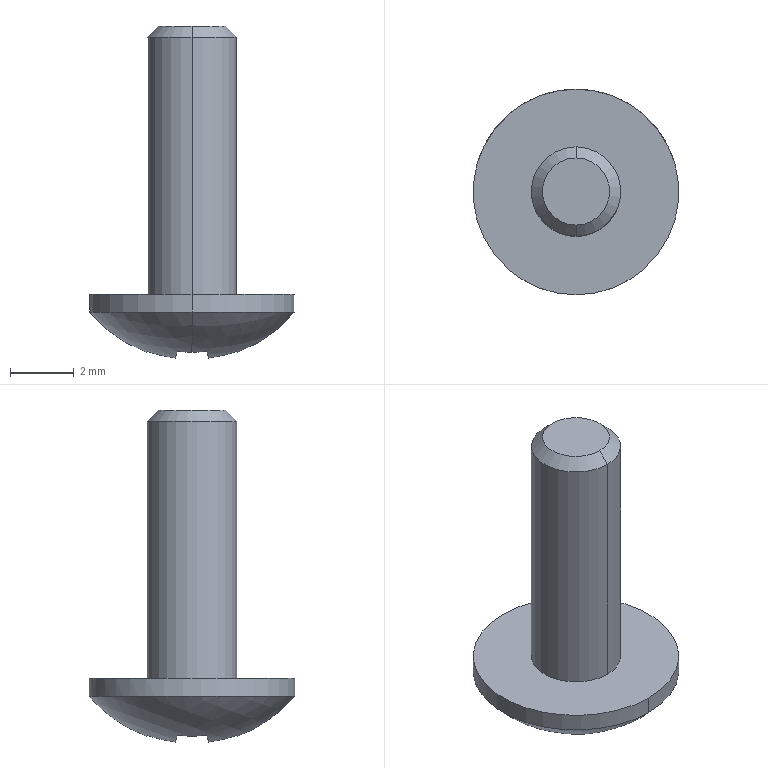Part | STEP file | MSBR-15XIAO_2_1_1_1 | 1 solid | 23 faces | box 6.44 x 6.44 x 10.399 mm | volume 92.165 mm3 | plane 15 | cylinder 4 | sphere 2 | cone 2 | commonest cylinder face diameters 2.8 x2 6.44 x2
STEP:
#1=CARTESIAN_POINT('',(0.,0.,0.));
#2=DIRECTION('',(0.,0.,1.));
#3=DIRECTION('',(1.,0.,0.));
#4=AXIS2_PLACEMENT_3D('',#1,#2,#3);
#5=CARTESIAN_POINT('',(0.,3.22,-13.09));
#6=VERTEX_POINT('',#5);
#7=CARTESIAN_POINT('',(0.,-3.22,-13.09));
#8=VERTEX_POINT('',#7);
#9=CARTESIAN_POINT('',(0.,0.,-13.09));
#10=DIRECTION('',(0.,0.,-1.));
#11=DIRECTION('',(0.,1.,0.));
#12=AXIS2_PLACEMENT_3D('',#9,#10,#11);
#13=CIRCLE('',#12,3.22);
#14=EDGE_CURVE('',#6,#8,#13,.T.);
#15=ORIENTED_EDGE('',*,*,#14,.F.);
#16=CARTESIAN_POINT('',(0.,3.22,-13.65));
#17=VERTEX_POINT('',#16);
#18=CARTESIAN_POINT('',(0.,3.22,-13.65));
#19=DIRECTION('',(0.,-0.000000001,1.));
#20=VECTOR('',#19,0.56);
#21=LINE('',#18,#20);
#22=EDGE_CURVE('',#17,#6,#21,.T.);
#23=ORIENTED_EDGE('',*,*,#22,.F.);
#24=CARTESIAN_POINT('',(0.,-3.22,-13.65));
#25=VERTEX_POINT('',#24);
#26=CARTESIAN_POINT('',(0.,0.,-13.65));
#27=DIRECTION('',(0.,0.,1.));
#28=DIRECTION('',(0.,-1.,0.));
#29=AXIS2_PLACEMENT_3D('',#26,#27,#28);
#30=CIRCLE('',#29,3.22);
#31=EDGE_CURVE('',#25,#17,#30,.T.);
#32=ORIENTED_EDGE('',*,*,#31,.F.);
#33=CARTESIAN_POINT('',(0.,-3.22,-13.09));
#34=DIRECTION('',(0.,-0.000000001,-1.));
#35=VECTOR('',#34,0.56);
#36=LINE('',#33,#35);
#37=EDGE_CURVE('',#8,#25,#36,.T.);
#38=ORIENTED_EDGE('',*,*,#37,.F.);
#39=EDGE_LOOP('',(#15,#23,#32,#38));
#40=FACE_OUTER_BOUND('',#39,.F.);
#41=CARTESIAN_POINT('',(0.,0.,-13.073));
#42=DIRECTION('',(0.,0.,-1.));
#43=DIRECTION('',(0.,1.,0.));
#44=AXIS2_PLACEMENT_3D('',#41,#42,#43);
#45=CYLINDRICAL_SURFACE('',#44,3.22);
#46=ADVANCED_FACE('',(#40),#45,.T.);
#47=CARTESIAN_POINT('',(0.,0.,-13.09));
#48=DIRECTION('',(0.,0.,-1.));
#49=DIRECTION('',(0.,-1.,0.));
#50=AXIS2_PLACEMENT_3D('',#47,#48,#49);
#51=CIRCLE('',#50,3.22);
#52=EDGE_CURVE('',#8,#6,#51,.T.);
#53=ORIENTED_EDGE('',*,*,#52,.T.);
#54=ORIENTED_EDGE('',*,*,#14,.T.);
#55=EDGE_LOOP('',(#53,#54));
#56=FACE_OUTER_BOUND('',#55,.F.);
#57=CARTESIAN_POINT('',(0.,-1.4,-13.09));
#58=VERTEX_POINT('',#57);
#59=CARTESIAN_POINT('',(0.,1.4,-13.09));
#60=VERTEX_POINT('',#59);
#61=CARTESIAN_POINT('',(0.,0.,-13.09));
#62=DIRECTION('',(0.,0.,1.));
#63=DIRECTION('',(0.,-1.,0.));
#64=AXIS2_PLACEMENT_3D('',#61,#62,#63);
#65=CIRCLE('',#64,1.4);
#66=EDGE_CURVE('',#58,#60,#65,.T.);
#67=ORIENTED_EDGE('',*,*,#66,.T.);
#68=CARTESIAN_POINT('',(0.,0.,-13.09));
#69=DIRECTION('',(0.,0.,1.));
#70=DIRECTION('',(0.,1.,0.));
#71=AXIS2_PLACEMENT_3D('',#68,#69,#70);
#72=CIRCLE('',#71,1.4);
#73=EDGE_CURVE('',#60,#58,#72,.T.);
#74=ORIENTED_EDGE('',*,*,#73,.T.);
#75=EDGE_LOOP('',(#67,#74));
#76=FACE_BOUND('',#75,.F.);
#77=CARTESIAN_POINT('',(0.,0.,-13.09));
#78=DIRECTION('',(0.,0.,1.));
#79=DIRECTION('',(0.,-1.,0.));
#80=AXIS2_PLACEMENT_3D('',#77,#78,#79);
#81=PLANE('',#80);
#82=ADVANCED_FACE('',(#56,#76),#81,.T.);
#83=ORIENTED_EDGE('',*,*,#37,.T.);
#84=CARTESIAN_POINT('',(0.,0.,-13.65));
#85=DIRECTION('',(0.,0.,1.));
#86=DIRECTION('',(0.,1.,0.));
#87=AXIS2_PLACEMENT_3D('',#84,#85,#86);
#88=CIRCLE('',#87,3.22);
#89=EDGE_CURVE('',#17,#25,#88,.T.);
#90=ORIENTED_EDGE('',*,*,#89,.F.);
#91=ORIENTED_EDGE('',*,*,#22,.T.);
#92=ORIENTED_EDGE('',*,*,#52,.F.);
#93=EDGE_LOOP('',(#83,#90,#91,#92));
#94=FACE_OUTER_BOUND('',#93,.F.);
#95=CARTESIAN_POINT('',(0.,0.,-13.073));
#96=DIRECTION('',(0.,0.,-1.));
#97=DIRECTION('',(0.,-1.,0.));
#98=AXIS2_PLACEMENT_3D('',#95,#96,#97);
#99=CYLINDRICAL_SURFACE('',#98,3.22);
#100=ADVANCED_FACE('',(#94),#99,.T.);
#101=ORIENTED_EDGE('',*,*,#89,.T.);
#102=CARTESIAN_POINT('',(0.,-1.421,-14.906));
#103=VERTEX_POINT('',#102);
#104=CARTESIAN_POINT('',(0.,0.,-10.953));
#105=DIRECTION('',(-1.,0.,0.));
#106=DIRECTION('',(0.,-0.3383,-0.941));
#107=AXIS2_PLACEMENT_3D('',#104,#105,#106);
#108=CIRCLE('',#107,4.2);
#109=EDGE_CURVE('',#103,#25,#108,.T.);
#110=ORIENTED_EDGE('',*,*,#109,.F.);
#111=CARTESIAN_POINT('',(-0.4683,-1.405,-14.884));
#112=VERTEX_POINT('',#111);
#113=CARTESIAN_POINT('',(0.,0.9385,-11.629));
#114=DIRECTION('',(0.,-0.8115,0.5843));
#115=DIRECTION('',(-0.116,-0.5804,-0.8061));
#116=AXIS2_PLACEMENT_3D('',#113,#114,#115);
#117=CIRCLE('',#116,4.038);
#118=EDGE_CURVE('',#112,#103,#117,.T.);
#119=ORIENTED_EDGE('',*,*,#118,.F.);
#120=CARTESIAN_POINT('',(-0.5176,-0.5176,-15.089));
#121=VERTEX_POINT('',#120);
#122=CARTESIAN_POINT('',(0.4491,0.,-11.061));
#123=DIRECTION('',(-0.9724,0.,0.2334));
#124=DIRECTION('',(-0.2316,-0.124,-0.9649));
#125=AXIS2_PLACEMENT_3D('',#122,#123,#124);
#126=CIRCLE('',#125,4.175);
#127=EDGE_CURVE('',#121,#112,#126,.T.);
#128=ORIENTED_EDGE('',*,*,#127,.F.);
#129=CARTESIAN_POINT('',(-1.405,-0.4683,-14.884));
#130=VERTEX_POINT('',#129);
#131=CARTESIAN_POINT('',(0.,0.4491,-11.061));
#132=DIRECTION('',(0.,-0.9724,0.2334));
#133=DIRECTION('',(-0.3365,-0.2198,-0.9157));
#134=AXIS2_PLACEMENT_3D('',#131,#132,#133);
#135=CIRCLE('',#134,4.175);
#136=EDGE_CURVE('',#130,#121,#135,.T.);
#137=ORIENTED_EDGE('',*,*,#136,.F.);
#138=CARTESIAN_POINT('',(-1.405,0.4683,-14.884));
#139=VERTEX_POINT('',#138);
#140=CARTESIAN_POINT('',(0.9385,0.,-11.629));
#141=DIRECTION('',(-0.8115,0.,0.5843));
#142=DIRECTION('',(-0.5804,0.116,-0.8061));
#143=AXIS2_PLACEMENT_3D('',#140,#141,#142);
#144=CIRCLE('',#143,4.038);
#145=EDGE_CURVE('',#139,#130,#144,.T.);
#146=ORIENTED_EDGE('',*,*,#145,.F.);
#147=CARTESIAN_POINT('',(-0.5176,0.5176,-15.089));
#148=VERTEX_POINT('',#147);
#149=CARTESIAN_POINT('',(0.,-0.4491,-11.061));
#150=DIRECTION('',(0.,-0.9724,-0.2334));
#151=DIRECTION('',(-0.3365,0.2198,-0.9157));
#152=AXIS2_PLACEMENT_3D('',#149,#150,#151);
#153=CIRCLE('',#152,4.175);
#154=EDGE_CURVE('',#139,#148,#153,.T.);
#155=ORIENTED_EDGE('',*,*,#154,.T.);
#156=CARTESIAN_POINT('',(-0.4683,1.405,-14.884));
#157=VERTEX_POINT('',#156);
#158=CARTESIAN_POINT('',(0.4491,0.,-11.061));
#159=DIRECTION('',(0.9724,0.,-0.2334));
#160=DIRECTION('',(-0.2316,0.124,-0.9649));
#161=AXIS2_PLACEMENT_3D('',#158,#159,#160);
#162=CIRCLE('',#161,4.175);
#163=EDGE_CURVE('',#148,#157,#162,.T.);
#164=ORIENTED_EDGE('',*,*,#163,.T.);
#165=CARTESIAN_POINT('',(0.,1.421,-14.906));
#166=VERTEX_POINT('',#165);
#167=CARTESIAN_POINT('',(0.,-0.9385,-11.629));
#168=DIRECTION('',(0.,0.8115,0.5843));
#169=DIRECTION('',(0.,0.5843,-0.8115));
#170=AXIS2_PLACEMENT_3D('',#167,#168,#169);
#171=CIRCLE('',#170,4.038);
#172=EDGE_CURVE('',#166,#157,#171,.T.);
#173=ORIENTED_EDGE('',*,*,#172,.F.);
#174=CARTESIAN_POINT('',(0.,0.,-10.953));
#175=DIRECTION('',(-1.,0.,0.));
#176=DIRECTION('',(0.,0.7667,-0.642));
#177=AXIS2_PLACEMENT_3D('',#174,#175,#176);
#178=CIRCLE('',#177,4.2);
#179=EDGE_CURVE('',#17,#166,#178,.T.);
#180=ORIENTED_EDGE('',*,*,#179,.F.);
#181=EDGE_LOOP('',(#101,#110,#119,#128,#137,#146,#155,#164,#173,#180));
#182=FACE_OUTER_BOUND('',#181,.F.);
#183=CARTESIAN_POINT('',(0.,0.,-10.953));
#184=DIRECTION('',(0.,0.3383,-0.941));
#185=DIRECTION('',(0.,-0.941,-0.3383));
#186=AXIS2_PLACEMENT_3D('',#183,#184,#185);
#187=SPHERICAL_SURFACE('',#186,4.2);
#188=ADVANCED_FACE('',(#182),#187,.T.);
#189=ORIENTED_EDGE('',*,*,#179,.T.);
#190=CARTESIAN_POINT('',(0.4683,1.405,-14.884));
#191=VERTEX_POINT('',#190);
#192=CARTESIAN_POINT('',(0.,-0.9385,-11.629));
#193=DIRECTION('',(0.,0.8115,0.5843));
#194=DIRECTION('',(0.116,0.5804,-0.8061));
#195=AXIS2_PLACEMENT_3D('',#192,#193,#194);
#196=CIRCLE('',#195,4.038);
#197=EDGE_CURVE('',#191,#166,#196,.T.);
#198=ORIENTED_EDGE('',*,*,#197,.F.);
#199=CARTESIAN_POINT('',(0.5176,0.5176,-15.089));
#200=VERTEX_POINT('',#199);
#201=CARTESIAN_POINT('',(-0.4491,0.,-11.061));
#202=DIRECTION('',(-0.9724,0.,-0.2334));
#203=DIRECTION('',(0.2198,0.3365,-0.9157));
#204=AXIS2_PLACEMENT_3D('',#201,#202,#203);
#205=CIRCLE('',#204,4.175);
#206=EDGE_CURVE('',#191,#200,#205,.T.);
#207=ORIENTED_EDGE('',*,*,#206,.T.);
#208=CARTESIAN_POINT('',(1.405,0.4683,-14.884));
#209=VERTEX_POINT('',#208);
#210=CARTESIAN_POINT('',(0.,-0.4491,-11.061));
#211=DIRECTION('',(0.,-0.9724,-0.2334));
#212=DIRECTION('',(0.124,0.2316,-0.9649));
#213=AXIS2_PLACEMENT_3D('',#210,#211,#212);
#214=CIRCLE('',#213,4.175);
#215=EDGE_CURVE('',#200,#209,#214,.T.);
#216=ORIENTED_EDGE('',*,*,#215,.T.);
#217=CARTESIAN_POINT('',(1.405,-0.4683,-14.884));
#218=VERTEX_POINT('',#217);
#219=CARTESIAN_POINT('',(-0.9385,0.,-11.629));
#220=DIRECTION('',(-0.8115,0.,-0.5843));
#221=DIRECTION('',(0.5804,0.116,-0.8061));
#222=AXIS2_PLACEMENT_3D('',#219,#220,#221);
#223=CIRCLE('',#222,4.038);
#224=EDGE_CURVE('',#209,#218,#223,.T.);
#225=ORIENTED_EDGE('',*,*,#224,.T.);
#226=CARTESIAN_POINT('',(0.5176,-0.5176,-15.089));
#227=VERTEX_POINT('',#226);
#228=CARTESIAN_POINT('',(0.,0.4491,-11.061));
#229=DIRECTION('',(0.,-0.9724,0.2334));
#230=DIRECTION('',(0.124,-0.2316,-0.9649));
#231=AXIS2_PLACEMENT_3D('',#228,#229,#230);
#232=CIRCLE('',#231,4.175);
#233=EDGE_CURVE('',#227,#218,#232,.T.);
#234=ORIENTED_EDGE('',*,*,#233,.F.);
#235=CARTESIAN_POINT('',(0.4683,-1.405,-14.884));
#236=VERTEX_POINT('',#235);
#237=CARTESIAN_POINT('',(-0.4491,0.,-11.061));
#238=DIRECTION('',(0.9724,0.,0.2334));
#239=DIRECTION('',(0.2198,-0.3365,-0.9157));
#240=AXIS2_PLACEMENT_3D('',#237,#238,#239);
#241=CIRCLE('',#240,4.175);
#242=EDGE_CURVE('',#236,#227,#241,.T.);
#243=ORIENTED_EDGE('',*,*,#242,.F.);
#244=CARTESIAN_POINT('',(0.,0.9385,-11.629));
#245=DIRECTION('',(0.,-0.8115,0.5843));
#246=DIRECTION('',(0.,-0.5843,-0.8115));
#247=AXIS2_PLACEMENT_3D('',#244,#245,#246);
#248=CIRCLE('',#247,4.038);
#249=EDGE_CURVE('',#103,#236,#248,.T.);
#250=ORIENTED_EDGE('',*,*,#249,.F.);
#251=ORIENTED_EDGE('',*,*,#109,.T.);
#252=ORIENTED_EDGE('',*,*,#31,.T.);
#253=EDGE_LOOP('',(#189,#198,#207,#216,#225,#234,#243,#250,#251,#252));
#254=FACE_OUTER_BOUND('',#253,.F.);
#255=CARTESIAN_POINT('',(0.,0.,-10.953));
#256=DIRECTION('',(0.,0.3383,-0.941));
#257=DIRECTION('',(0.,0.941,0.3383));
#258=AXIS2_PLACEMENT_3D('',#255,#256,#257);
#259=SPHERICAL_SURFACE('',#258,4.2);
#260=ADVANCED_FACE('',(#254),#259,.T.);
#261=CARTESIAN_POINT('',(0.105,0.315,-13.37));
#262=VERTEX_POINT('',#261);
#263=CARTESIAN_POINT('',(0.4683,1.405,-14.884));
#264=DIRECTION('',(-0.1912,-0.5735,0.7966));
#265=VECTOR('',#264,1.9);
#266=LINE('',#263,#265);
#267=EDGE_CURVE('',#191,#262,#266,.T.);
#268=ORIENTED_EDGE('',*,*,#267,.F.);
#269=ORIENTED_EDGE('',*,*,#197,.T.);
#270=ORIENTED_EDGE('',*,*,#172,.T.);
#271=CARTESIAN_POINT('',(-0.105,0.315,-13.37));
#272=VERTEX_POINT('',#271);
#273=CARTESIAN_POINT('',(-0.105,0.315,-13.37));
#274=DIRECTION('',(-0.1912,0.5735,-0.7966));
#275=VECTOR('',#274,1.9);
#276=LINE('',#273,#275);
#277=EDGE_CURVE('',#272,#157,#276,.T.);
#278=ORIENTED_EDGE('',*,*,#277,.F.);
#279=CARTESIAN_POINT('',(0.105,0.315,-13.37));
#280=DIRECTION('',(-1.,0.,0.));
#281=VECTOR('',#280,0.21);
#282=LINE('',#279,#281);
#283=EDGE_CURVE('',#262,#272,#282,.T.);
#284=ORIENTED_EDGE('',*,*,#283,.F.);
#285=EDGE_LOOP('',(#268,#269,#270,#278,#284));
#286=FACE_OUTER_BOUND('',#285,.F.);
#287=CARTESIAN_POINT('',(0.,0.8679,-14.138));
#288=DIRECTION('',(0.,0.8115,0.5843));
#289=DIRECTION('',(1.,0.,0.));
#290=AXIS2_PLACEMENT_3D('',#287,#288,#289);
#291=PLANE('',#290);
#292=ADVANCED_FACE('',(#286),#291,.F.);
#293=CARTESIAN_POINT('',(0.105,0.105,-13.37));
#294=VERTEX_POINT('',#293);
#295=CARTESIAN_POINT('',(0.105,0.105,-13.37));
#296=DIRECTION('',(0.,1.,0.));
#297=VECTOR('',#296,0.21);
#298=LINE('',#295,#297);
#299=EDGE_CURVE('',#294,#262,#298,.T.);
#300=ORIENTED_EDGE('',*,*,#299,.F.);
#301=CARTESIAN_POINT('',(0.5176,0.5176,-15.089));
#302=DIRECTION('',(-0.2273,-0.2273,0.9469));
#303=VECTOR('',#302,1.815);
#304=LINE('',#301,#303);
#305=EDGE_CURVE('',#200,#294,#304,.T.);
#306=ORIENTED_EDGE('',*,*,#305,.F.);
#307=ORIENTED_EDGE('',*,*,#206,.F.);
#308=ORIENTED_EDGE('',*,*,#267,.T.);
#309=EDGE_LOOP('',(#300,#306,#307,#308));
#310=FACE_OUTER_BOUND('',#309,.F.);
#311=CARTESIAN_POINT('',(0.3113,0.7549,-14.23));
#312=DIRECTION('',(0.9724,0.,0.2334));
#313=DIRECTION('',(0.,-1.,0.));
#314=AXIS2_PLACEMENT_3D('',#311,#312,#313);
#315=PLANE('',#314);
#316=ADVANCED_FACE('',(#310),#315,.F.);
#317=CARTESIAN_POINT('',(-0.315,0.105,-13.37));
#318=VERTEX_POINT('',#317);
#319=CARTESIAN_POINT('',(-0.105,0.105,-13.37));
#320=VERTEX_POINT('',#319);
#321=CARTESIAN_POINT('',(-0.315,0.105,-13.37));
#322=DIRECTION('',(1.,0.,0.));
#323=VECTOR('',#322,0.21);
#324=LINE('',#321,#323);
#325=EDGE_CURVE('',#318,#320,#324,.T.);
#326=ORIENTED_EDGE('',*,*,#325,.F.);
#327=CARTESIAN_POINT('',(-0.315,-0.105,-13.37));
#328=VERTEX_POINT('',#327);
#329=CARTESIAN_POINT('',(-0.315,-0.105,-13.37));
#330=DIRECTION('',(0.,1.,0.));
#331=VECTOR('',#330,0.21);
#332=LINE('',#329,#331);
#333=EDGE_CURVE('',#328,#318,#332,.T.);
#334=ORIENTED_EDGE('',*,*,#333,.F.);
#335=CARTESIAN_POINT('',(-0.105,-0.105,-13.37));
#336=VERTEX_POINT('',#335);
#337=CARTESIAN_POINT('',(-0.105,-0.105,-13.37));
#338=DIRECTION('',(-1.,0.,0.));
#339=VECTOR('',#338,0.21);
#340=LINE('',#337,#339);
#341=EDGE_CURVE('',#336,#328,#340,.T.);
#342=ORIENTED_EDGE('',*,*,#341,.F.);
#343=CARTESIAN_POINT('',(-0.105,-0.315,-13.37));
#344=VERTEX_POINT('',#343);
#345=CARTESIAN_POINT('',(-0.105,-0.315,-13.37));
#346=DIRECTION('',(0.,1.,0.));
#347=VECTOR('',#346,0.21);
#348=LINE('',#345,#347);
#349=EDGE_CURVE('',#344,#336,#348,.T.);
#350=ORIENTED_EDGE('',*,*,#349,.F.);
#351=CARTESIAN_POINT('',(0.105,-0.315,-13.37));
#352=VERTEX_POINT('',#351);
#353=CARTESIAN_POINT('',(0.105,-0.315,-13.37));
#354=DIRECTION('',(-1.,0.,0.));
#355=VECTOR('',#354,0.21);
#356=LINE('',#353,#355);
#357=EDGE_CURVE('',#352,#344,#356,.T.);
#358=ORIENTED_EDGE('',*,*,#357,.F.);
#359=CARTESIAN_POINT('',(0.105,-0.105,-13.37));
#360=VERTEX_POINT('',#359);
#361=CARTESIAN_POINT('',(0.105,-0.105,-13.37));
#362=DIRECTION('',(0.,-1.,0.));
#363=VECTOR('',#362,0.21);
#364=LINE('',#361,#363);
#365=EDGE_CURVE('',#360,#352,#364,.T.);
#366=ORIENTED_EDGE('',*,*,#365,.F.);
#367=CARTESIAN_POINT('',(0.315,-0.105,-13.37));
#368=VERTEX_POINT('',#367);
#369=CARTESIAN_POINT('',(0.315,-0.105,-13.37));
#370=DIRECTION('',(-1.,0.,0.));
#371=VECTOR('',#370,0.21);
#372=LINE('',#369,#371);
#373=EDGE_CURVE('',#368,#360,#372,.T.);
#374=ORIENTED_EDGE('',*,*,#373,.F.);
#375=CARTESIAN_POINT('',(0.315,0.105,-13.37));
#376=VERTEX_POINT('',#375);
#377=CARTESIAN_POINT('',(0.315,0.105,-13.37));
#378=DIRECTION('',(0.,-1.,0.));
#379=VECTOR('',#378,0.21);
#380=LINE('',#377,#379);
#381=EDGE_CURVE('',#376,#368,#380,.T.);
#382=ORIENTED_EDGE('',*,*,#381,.F.);
#383=CARTESIAN_POINT('',(0.105,0.105,-13.37));
#384=DIRECTION('',(1.,0.,0.));
#385=VECTOR('',#384,0.21);
#386=LINE('',#383,#385);
#387=EDGE_CURVE('',#294,#376,#386,.T.);
#388=ORIENTED_EDGE('',*,*,#387,.F.);
#389=ORIENTED_EDGE('',*,*,#299,.T.);
#390=ORIENTED_EDGE('',*,*,#283,.T.);
#391=CARTESIAN_POINT('',(-0.105,0.105,-13.37));
#392=DIRECTION('',(0.,1.,0.));
#393=VECTOR('',#392,0.21);
#394=LINE('',#391,#393);
#395=EDGE_CURVE('',#320,#272,#394,.T.);
#396=ORIENTED_EDGE('',*,*,#395,.F.);
#397=EDGE_LOOP('',(#326,#334,#342,#350,#358,#366,#374,#382,#388,#389,#390,#396));
#398=FACE_OUTER_BOUND('',#397,.F.);
#399=CARTESIAN_POINT('',(0.,0.,-13.37));
#400=DIRECTION('',(0.,0.,1.));
#401=DIRECTION('',(0.,-1.,0.));
#402=AXIS2_PLACEMENT_3D('',#399,#400,#401);
#403=PLANE('',#402);
#404=ADVANCED_FACE('',(#398),#403,.F.);
#405=ORIENTED_EDGE('',*,*,#325,.T.);
#406=CARTESIAN_POINT('',(-0.5176,0.5176,-15.089));
#407=DIRECTION('',(0.2273,-0.2273,0.9469));
#408=VECTOR('',#407,1.815);
#409=LINE('',#406,#408);
#410=EDGE_CURVE('',#148,#320,#409,.T.);
#411=ORIENTED_EDGE('',*,*,#410,.F.);
#412=ORIENTED_EDGE('',*,*,#154,.F.);
#413=CARTESIAN_POINT('',(-0.315,0.105,-13.37));
#414=DIRECTION('',(-0.5735,0.1912,-0.7966));
#415=VECTOR('',#414,1.9);
#416=LINE('',#413,#415);
#417=EDGE_CURVE('',#318,#139,#416,.T.);
#418=ORIENTED_EDGE('',*,*,#417,.F.);
#419=EDGE_LOOP('',(#405,#411,#412,#418));
#420=FACE_OUTER_BOUND('',#419,.F.);
#421=CARTESIAN_POINT('',(-0.7549,0.3113,-14.23));
#422=DIRECTION('',(0.,0.9724,0.2334));
#423=DIRECTION('',(1.,0.,0.));
#424=AXIS2_PLACEMENT_3D('',#421,#422,#423);
#425=PLANE('',#424);
#426=ADVANCED_FACE('',(#420),#425,.F.);
#427=ORIENTED_EDGE('',*,*,#395,.T.);
#428=ORIENTED_EDGE('',*,*,#277,.T.);
#429=ORIENTED_EDGE('',*,*,#163,.F.);
#430=ORIENTED_EDGE('',*,*,#410,.T.);
#431=EDGE_LOOP('',(#427,#428,#429,#430));
#432=FACE_OUTER_BOUND('',#431,.F.);
#433=CARTESIAN_POINT('',(-0.3113,0.7549,-14.23));
#434=DIRECTION('',(0.9724,0.,-0.2334));
#435=DIRECTION('',(0.,1.,0.));
#436=AXIS2_PLACEMENT_3D('',#433,#434,#435);
#437=PLANE('',#436);
#438=ADVANCED_FACE('',(#432),#437,.T.);
#439=ORIENTED_EDGE('',*,*,#333,.T.);
#440=ORIENTED_EDGE('',*,*,#417,.T.);
#441=ORIENTED_EDGE('',*,*,#145,.T.);
#442=CARTESIAN_POINT('',(-0.315,-0.105,-13.37));
#443=DIRECTION('',(-0.5735,-0.1912,-0.7966));
#444=VECTOR('',#443,1.9);
#445=LINE('',#442,#444);
#446=EDGE_CURVE('',#328,#130,#445,.T.);
#447=ORIENTED_EDGE('',*,*,#446,.F.);
#448=EDGE_LOOP('',(#439,#440,#441,#447));
#449=FACE_OUTER_BOUND('',#448,.F.);
#450=CARTESIAN_POINT('',(-0.8679,0.,-14.138));
#451=DIRECTION('',(0.8115,0.,-0.5843));
#452=DIRECTION('',(0.,1.,0.));
#453=AXIS2_PLACEMENT_3D('',#450,#451,#452);
#454=PLANE('',#453);
#455=ADVANCED_FACE('',(#449),#454,.T.);
#456=ORIENTED_EDGE('',*,*,#341,.T.);
#457=ORIENTED_EDGE('',*,*,#446,.T.);
#458=ORIENTED_EDGE('',*,*,#136,.T.);
#459=CARTESIAN_POINT('',(-0.105,-0.105,-13.37));
#460=DIRECTION('',(-0.2273,-0.2273,-0.9469));
#461=VECTOR('',#460,1.815);
#462=LINE('',#459,#461);
#463=EDGE_CURVE('',#336,#121,#462,.T.);
#464=ORIENTED_EDGE('',*,*,#463,.F.);
#465=EDGE_LOOP('',(#456,#457,#458,#464));
#466=FACE_OUTER_BOUND('',#465,.F.);
#467=CARTESIAN_POINT('',(-0.7549,-0.3113,-14.23));
#468=DIRECTION('',(0.,0.9724,-0.2334));
#469=DIRECTION('',(-1.,0.,0.));
#470=AXIS2_PLACEMENT_3D('',#467,#468,#469);
#471=PLANE('',#470);
#472=ADVANCED_FACE('',(#466),#471,.T.);
#473=ORIENTED_EDGE('',*,*,#349,.T.);
#474=ORIENTED_EDGE('',*,*,#463,.T.);
#475=ORIENTED_EDGE('',*,*,#127,.T.);
#476=CARTESIAN_POINT('',(-0.105,-0.315,-13.37));
#477=DIRECTION('',(-0.1912,-0.5735,-0.7966));
#478=VECTOR('',#477,1.9);
#479=LINE('',#476,#478);
#480=EDGE_CURVE('',#344,#112,#479,.T.);
#481=ORIENTED_EDGE('',*,*,#480,.F.);
#482=EDGE_LOOP('',(#473,#474,#475,#481));
#483=FACE_OUTER_BOUND('',#482,.F.);
#484=CARTESIAN_POINT('',(-0.3113,-0.7549,-14.23));
#485=DIRECTION('',(0.9724,0.,-0.2334));
#486=DIRECTION('',(0.,1.,0.));
#487=AXIS2_PLACEMENT_3D('',#484,#485,#486);
#488=PLANE('',#487);
#489=ADVANCED_FACE('',(#483),#488,.T.);
#490=ORIENTED_EDGE('',*,*,#357,.T.);
#491=ORIENTED_EDGE('',*,*,#480,.T.);
#492=ORIENTED_EDGE('',*,*,#118,.T.);
#493=ORIENTED_EDGE('',*,*,#249,.T.);
#494=CARTESIAN_POINT('',(0.105,-0.315,-13.37));
#495=DIRECTION('',(0.1912,-0.5735,-0.7966));
#496=VECTOR('',#495,1.9);
#497=LINE('',#494,#496);
#498=EDGE_CURVE('',#352,#236,#497,.T.);
#499=ORIENTED_EDGE('',*,*,#498,.F.);
#500=EDGE_LOOP('',(#490,#491,#492,#493,#499));
#501=FACE_OUTER_BOUND('',#500,.F.);
#502=CARTESIAN_POINT('',(0.,-0.8679,-14.138));
#503=DIRECTION('',(0.,0.8115,-0.5843));
#504=DIRECTION('',(-1.,0.,0.));
#505=AXIS2_PLACEMENT_3D('',#502,#503,#504);
#506=PLANE('',#505);
#507=ADVANCED_FACE('',(#501),#506,.T.);
#508=ORIENTED_EDGE('',*,*,#365,.T.);
#509=ORIENTED_EDGE('',*,*,#498,.T.);
#510=ORIENTED_EDGE('',*,*,#242,.T.);
#511=CARTESIAN_POINT('',(0.105,-0.105,-13.37));
#512=DIRECTION('',(0.2273,-0.2273,-0.9469));
#513=VECTOR('',#512,1.815);
#514=LINE('',#511,#513);
#515=EDGE_CURVE('',#360,#227,#514,.T.);
#516=ORIENTED_EDGE('',*,*,#515,.F.);
#517=EDGE_LOOP('',(#508,#509,#510,#516));
#518=FACE_OUTER_BOUND('',#517,.F.);
#519=CARTESIAN_POINT('',(0.3113,-0.7549,-14.23));
#520=DIRECTION('',(0.9724,0.,0.2334));
#521=DIRECTION('',(0.,-1.,0.));
#522=AXIS2_PLACEMENT_3D('',#519,#520,#521);
#523=PLANE('',#522);
#524=ADVANCED_FACE('',(#518),#523,.F.);
#525=ORIENTED_EDGE('',*,*,#373,.T.);
#526=ORIENTED_EDGE('',*,*,#515,.T.);
#527=ORIENTED_EDGE('',*,*,#233,.T.);
#528=CARTESIAN_POINT('',(0.315,-0.105,-13.37));
#529=DIRECTION('',(0.5735,-0.1912,-0.7966));
#530=VECTOR('',#529,1.9);
#531=LINE('',#528,#530);
#532=EDGE_CURVE('',#368,#218,#531,.T.);
#533=ORIENTED_EDGE('',*,*,#532,.F.);
#534=EDGE_LOOP('',(#525,#526,#527,#533));
#535=FACE_OUTER_BOUND('',#534,.F.);
#536=CARTESIAN_POINT('',(0.7549,-0.3113,-14.23));
#537=DIRECTION('',(0.,0.9724,-0.2334));
#538=DIRECTION('',(-1.,0.,0.));
#539=AXIS2_PLACEMENT_3D('',#536,#537,#538);
#540=PLANE('',#539);
#541=ADVANCED_FACE('',(#535),#540,.T.);
#542=ORIENTED_EDGE('',*,*,#381,.T.);
#543=ORIENTED_EDGE('',*,*,#532,.T.);
#544=ORIENTED_EDGE('',*,*,#224,.F.);
#545=CARTESIAN_POINT('',(0.315,0.105,-13.37));
#546=DIRECTION('',(0.5735,0.1912,-0.7966));
#547=VECTOR('',#546,1.9);
#548=LINE('',#545,#547);
#549=EDGE_CURVE('',#376,#209,#548,.T.);
#550=ORIENTED_EDGE('',*,*,#549,.F.);
#551=EDGE_LOOP('',(#542,#543,#544,#550));
#552=FACE_OUTER_BOUND('',#551,.F.);
#553=CARTESIAN_POINT('',(0.8679,0.,-14.138));
#554=DIRECTION('',(0.8115,0.,0.5843));
#555=DIRECTION('',(0.,-1.,0.));
#556=AXIS2_PLACEMENT_3D('',#553,#554,#555);
#557=PLANE('',#556);
#558=ADVANCED_FACE('',(#552),#557,.F.);
#559=ORIENTED_EDGE('',*,*,#387,.T.);
#560=ORIENTED_EDGE('',*,*,#549,.T.);
#561=ORIENTED_EDGE('',*,*,#215,.F.);
#562=ORIENTED_EDGE('',*,*,#305,.T.);
#563=EDGE_LOOP('',(#559,#560,#561,#562));
#564=FACE_OUTER_BOUND('',#563,.F.);
#565=CARTESIAN_POINT('',(0.7549,0.3113,-14.23));
#566=DIRECTION('',(0.,0.9724,0.2334));
#567=DIRECTION('',(1.,0.,0.));
#568=AXIS2_PLACEMENT_3D('',#565,#566,#567);
#569=PLANE('',#568);
#570=ADVANCED_FACE('',(#564),#569,.F.);
#571=CARTESIAN_POINT('',(0.,1.4,-5.04));
#572=VERTEX_POINT('',#571);
#573=CARTESIAN_POINT('',(0.,-1.4,-5.04));
#574=VERTEX_POINT('',#573);
#575=CARTESIAN_POINT('',(0.,0.,-5.04));
#576=DIRECTION('',(0.000000001,0.,-1.));
#577=DIRECTION('',(0.,1.,0.));
#578=AXIS2_PLACEMENT_3D('',#575,#576,#577);
#579=CIRCLE('',#578,1.4);
#580=EDGE_CURVE('',#572,#574,#579,.T.);
#581=ORIENTED_EDGE('',*,*,#580,.F.);
#582=CARTESIAN_POINT('',(0.,1.4,-13.09));
#583=DIRECTION('',(0.,0.,1.));
#584=VECTOR('',#583,8.05);
#585=LINE('',#582,#584);
#586=EDGE_CURVE('',#60,#572,#585,.T.);
#587=ORIENTED_EDGE('',*,*,#586,.F.);
#588=ORIENTED_EDGE('',*,*,#66,.F.);
#589=CARTESIAN_POINT('',(0.,-1.4,-5.04));
#590=DIRECTION('',(0.,0.,-1.));
#591=VECTOR('',#590,8.05);
#592=LINE('',#589,#591);
#593=EDGE_CURVE('',#574,#58,#592,.T.);
#594=ORIENTED_EDGE('',*,*,#593,.F.);
#595=EDGE_LOOP('',(#581,#587,#588,#594));
#596=FACE_OUTER_BOUND('',#595,.F.);
#597=CARTESIAN_POINT('',(0.,0.,-4.879));
#598=DIRECTION('',(0.,0.,-1.));
#599=DIRECTION('',(0.,1.,0.));
#600=AXIS2_PLACEMENT_3D('',#597,#598,#599);
#601=CYLINDRICAL_SURFACE('',#600,1.4);
#602=ADVANCED_FACE('',(#596),#601,.T.);
#603=CARTESIAN_POINT('',(0.,1.05,-4.69));
#604=VERTEX_POINT('',#603);
#605=CARTESIAN_POINT('',(0.,-1.05,-4.69));
#606=VERTEX_POINT('',#605);
#607=CARTESIAN_POINT('',(0.,0.,-4.69));
#608=DIRECTION('',(0.000000001,0.,-1.));
#609=DIRECTION('',(0.,1.,0.));
#610=AXIS2_PLACEMENT_3D('',#607,#608,#609);
#611=CIRCLE('',#610,1.05);
#612=EDGE_CURVE('',#604,#606,#611,.T.);
#613=ORIENTED_EDGE('',*,*,#612,.F.);
#614=CARTESIAN_POINT('',(0.,1.4,-5.04));
#615=DIRECTION('',(0.,-0.7071,0.7071));
#616=VECTOR('',#615,0.495);
#617=LINE('',#614,#616);
#618=EDGE_CURVE('',#572,#604,#617,.T.);
#619=ORIENTED_EDGE('',*,*,#618,.F.);
#620=ORIENTED_EDGE('',*,*,#580,.T.);
#621=CARTESIAN_POINT('',(0.,-1.05,-4.69));
#622=DIRECTION('',(0.,-0.7071,-0.7071));
#623=VECTOR('',#622,0.495);
#624=LINE('',#621,#623);
#625=EDGE_CURVE('',#606,#574,#624,.T.);
#626=ORIENTED_EDGE('',*,*,#625,.F.);
#627=EDGE_LOOP('',(#613,#619,#620,#626));
#628=FACE_OUTER_BOUND('',#627,.F.);
#629=CARTESIAN_POINT('',(0.,0.,-4.865));
#630=DIRECTION('',(0.000000001,0.,-1.));
#631=DIRECTION('',(0.,-1.,0.));
#632=AXIS2_PLACEMENT_3D('',#629,#630,#631);
#633=CONICAL_SURFACE('',#632,1.225,45.);
#634=ADVANCED_FACE('',(#628),#633,.T.);
#635=CARTESIAN_POINT('',(0.,0.,-4.69));
#636=DIRECTION('',(-0.000000001,0.,-1.));
#637=DIRECTION('',(0.,-1.,0.));
#638=AXIS2_PLACEMENT_3D('',#635,#636,#637);
#639=CIRCLE('',#638,1.05);
#640=EDGE_CURVE('',#606,#604,#639,.T.);
#641=ORIENTED_EDGE('',*,*,#640,.T.);
#642=ORIENTED_EDGE('',*,*,#612,.T.);
#643=EDGE_LOOP('',(#641,#642));
#644=FACE_OUTER_BOUND('',#643,.F.);
#645=CARTESIAN_POINT('',(0.,0.,-4.69));
#646=DIRECTION('',(0.,0.,1.));
#647=DIRECTION('',(0.,-1.,0.));
#648=AXIS2_PLACEMENT_3D('',#645,#646,#647);
#649=PLANE('',#648);
#650=ADVANCED_FACE('',(#644),#649,.T.);
#651=ORIENTED_EDGE('',*,*,#625,.T.);
#652=CARTESIAN_POINT('',(0.,0.,-5.04));
#653=DIRECTION('',(-0.000000001,0.,-1.));
#654=DIRECTION('',(0.,-1.,0.));
#655=AXIS2_PLACEMENT_3D('',#652,#653,#654);
#656=CIRCLE('',#655,1.4);
#657=EDGE_CURVE('',#574,#572,#656,.T.);
#658=ORIENTED_EDGE('',*,*,#657,.T.);
#659=ORIENTED_EDGE('',*,*,#618,.T.);
#660=ORIENTED_EDGE('',*,*,#640,.F.);
#661=EDGE_LOOP('',(#651,#658,#659,#660));
#662=FACE_OUTER_BOUND('',#661,.F.);
#663=CARTESIAN_POINT('',(0.,0.,-4.865));
#664=DIRECTION('',(-0.000000001,0.,-1.));
#665=DIRECTION('',(0.,1.,0.));
#666=AXIS2_PLACEMENT_3D('',#663,#664,#665);
#667=CONICAL_SURFACE('',#666,1.225,45.);
#668=ADVANCED_FACE('',(#662),#667,.T.);
#669=ORIENTED_EDGE('',*,*,#593,.T.);
#670=ORIENTED_EDGE('',*,*,#73,.F.);
#671=ORIENTED_EDGE('',*,*,#586,.T.);
#672=ORIENTED_EDGE('',*,*,#657,.F.);
#673=EDGE_LOOP('',(#669,#670,#671,#672));
#674=FACE_OUTER_BOUND('',#673,.F.);
#675=CARTESIAN_POINT('',(0.,0.,-4.879));
#676=DIRECTION('',(0.,0.,-1.));
#677=DIRECTION('',(0.,-1.,0.));
#678=AXIS2_PLACEMENT_3D('',#675,#676,#677);
#679=CYLINDRICAL_SURFACE('',#678,1.4);
#680=ADVANCED_FACE('',(#674),#679,.T.);
#681=CLOSED_SHELL('',(#46,#82,#100,#188,#260,#292,#316,#404,#426,#438,#455,#472,#489,#507,#524,#541,#558,#570,#602,#634,#650,#668,#680));
#682=MANIFOLD_SOLID_BREP('',#681);
#683=(LENGTH_UNIT()NAMED_UNIT(*)SI_UNIT(.MILLI.,.METRE.));
#684=UNCERTAINTY_MEASURE_WITH_UNIT(LENGTH_MEASURE(0.001506),#683,'','');
#685=(NAMED_UNIT(*)PLANE_ANGLE_UNIT()SI_UNIT($,.RADIAN.));
#686=PLANE_ANGLE_MEASURE_WITH_UNIT(PLANE_ANGLE_MEASURE(0.01745),#685);
#687=(CONVERSION_BASED_UNIT('DEGREE',#686)NAMED_UNIT(*)PLANE_ANGLE_UNIT());
#688=(NAMED_UNIT(*)SI_UNIT($,.STERADIAN.)SOLID_ANGLE_UNIT());
#689=(GEOMETRIC_REPRESENTATION_CONTEXT(3)GLOBAL_UNCERTAINTY_ASSIGNED_CONTEXT((#684))GLOBAL_UNIT_ASSIGNED_CONTEXT((#683,#687,#688))REPRESENTATION_CONTEXT('',''));
#690=ADVANCED_BREP_SHAPE_REPRESENTATION('',(#4,#682),#689);